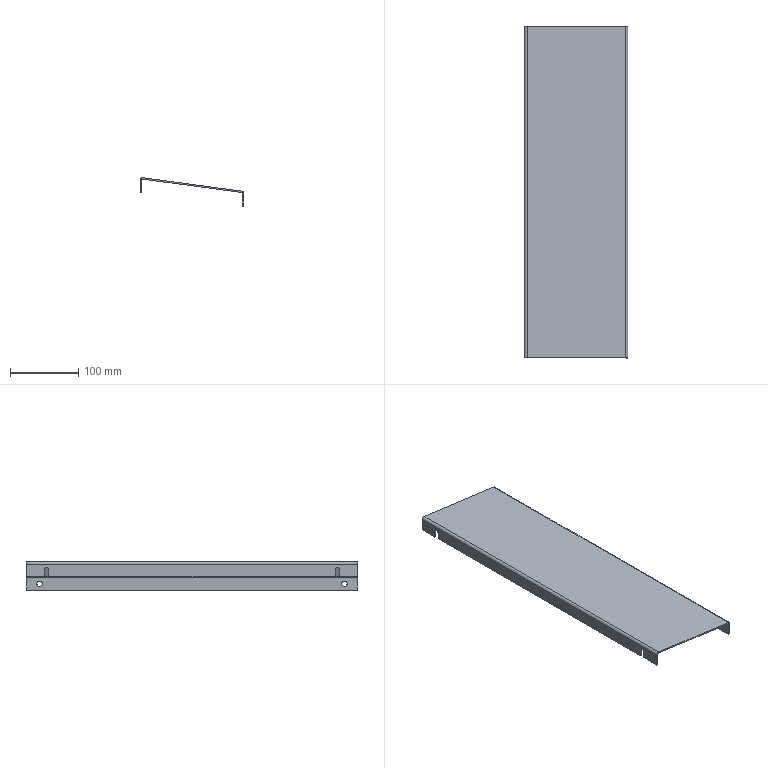Part | STEP file | JBJ-P-1006-08 | 1 solid | 32 faces | box 152 x 488 x 41.784 mm | volume 186030 mm3 | plane 24 | cylinder 8 | commonest cylinder face diameters 3 x2 6.5 x2 7 x2 8 x2
STEP:
#1=CARTESIAN_POINT('',(-2.,461.25,0.));
#2=VERTEX_POINT('',#1);
#3=CARTESIAN_POINT('',(0.,461.25,0.));
#4=VERTEX_POINT('',#3);
#5=CARTESIAN_POINT('',(-2.,461.25,0.));
#6=DIRECTION('',(1.,0.,0.));
#7=VECTOR('',#6,1000.);
#8=LINE('',#5,#7);
#9=EDGE_CURVE('',#2,#4,#8,.T.);
#10=ORIENTED_EDGE('',*,*,#9,.F.);
#11=CARTESIAN_POINT('',(-2.,488.,0.));
#12=VERTEX_POINT('',#11);
#13=CARTESIAN_POINT('',(-2.,488.,0.));
#14=DIRECTION('',(0.,-1.,0.));
#15=VECTOR('',#14,1000.);
#16=LINE('',#13,#15);
#17=EDGE_CURVE('',#12,#2,#16,.T.);
#18=ORIENTED_EDGE('',*,*,#17,.F.);
#19=CARTESIAN_POINT('',(0.,488.,0.));
#20=VERTEX_POINT('',#19);
#21=CARTESIAN_POINT('',(-2.,488.,0.));
#22=DIRECTION('',(1.,0.,0.));
#23=VECTOR('',#22,1000.);
#24=LINE('',#21,#23);
#25=EDGE_CURVE('',#12,#20,#24,.T.);
#26=ORIENTED_EDGE('',*,*,#25,.T.);
#27=CARTESIAN_POINT('',(0.,488.,0.));
#28=DIRECTION('',(0.,-1.,0.));
#29=VECTOR('',#28,1000.);
#30=LINE('',#27,#29);
#31=EDGE_CURVE('',#20,#4,#30,.T.);
#32=ORIENTED_EDGE('',*,*,#31,.T.);
#33=EDGE_LOOP('',(#10,#18,#26,#32));
#34=FACE_OUTER_BOUND('',#33,.T.);
#35=CARTESIAN_POINT('',(-2.,488.,0.));
#36=DIRECTION('',(0.,0.,-1.));
#37=DIRECTION('',(-1.,0.,0.));
#38=AXIS2_PLACEMENT_3D('',#35,#36,#37);
#39=PLANE('',#38);
#40=ADVANCED_FACE('',(#34),#39,.T.);
#41=CARTESIAN_POINT('',(0.,454.75,0.));
#42=VERTEX_POINT('',#41);
#43=CARTESIAN_POINT('',(-2.,454.75,0.));
#44=VERTEX_POINT('',#43);
#45=CARTESIAN_POINT('',(-2.,454.75,0.));
#46=DIRECTION('',(-1.,0.,0.));
#47=VECTOR('',#46,1000.);
#48=LINE('',#45,#47);
#49=EDGE_CURVE('',#42,#44,#48,.T.);
#50=ORIENTED_EDGE('',*,*,#49,.F.);
#51=CARTESIAN_POINT('',(0.,33.25,0.));
#52=VERTEX_POINT('',#51);
#53=CARTESIAN_POINT('',(0.,488.,0.));
#54=DIRECTION('',(0.,-1.,0.));
#55=VECTOR('',#54,1000.);
#56=LINE('',#53,#55);
#57=EDGE_CURVE('',#42,#52,#56,.T.);
#58=ORIENTED_EDGE('',*,*,#57,.T.);
#59=CARTESIAN_POINT('',(-2.,33.25,0.));
#60=VERTEX_POINT('',#59);
#61=CARTESIAN_POINT('',(-2.,33.25,0.));
#62=DIRECTION('',(1.,0.,0.));
#63=VECTOR('',#62,1000.);
#64=LINE('',#61,#63);
#65=EDGE_CURVE('',#60,#52,#64,.T.);
#66=ORIENTED_EDGE('',*,*,#65,.F.);
#67=CARTESIAN_POINT('',(-2.,488.,0.));
#68=DIRECTION('',(0.,-1.,0.));
#69=VECTOR('',#68,1000.);
#70=LINE('',#67,#69);
#71=EDGE_CURVE('',#44,#60,#70,.T.);
#72=ORIENTED_EDGE('',*,*,#71,.F.);
#73=EDGE_LOOP('',(#50,#58,#66,#72));
#74=FACE_OUTER_BOUND('',#73,.T.);
#75=CARTESIAN_POINT('',(-2.,488.,0.));
#76=DIRECTION('',(0.,0.,-1.));
#77=DIRECTION('',(-1.,0.,0.));
#78=AXIS2_PLACEMENT_3D('',#75,#76,#77);
#79=PLANE('',#78);
#80=ADVANCED_FACE('',(#74),#79,.T.);
#81=CARTESIAN_POINT('',(1.701,488.,19.77));
#82=VERTEX_POINT('',#81);
#83=CARTESIAN_POINT('',(1.969,488.,21.752));
#84=VERTEX_POINT('',#83);
#85=CARTESIAN_POINT('',(1.701,488.,19.77));
#86=DIRECTION('',(0.1339,0.,0.991));
#87=VECTOR('',#86,1000.);
#88=LINE('',#85,#87);
#89=EDGE_CURVE('',#82,#84,#88,.T.);
#90=ORIENTED_EDGE('',*,*,#89,.F.);
#91=CARTESIAN_POINT('',(0.,488.,18.284));
#92=VERTEX_POINT('',#91);
#93=CARTESIAN_POINT('',(1.5,488.,18.284));
#94=DIRECTION('',(0.,1.,0.));
#95=DIRECTION('',(0.,0.,-1.));
#96=AXIS2_PLACEMENT_3D('',#93,#94,#95);
#97=CIRCLE('',#96,1.5);
#98=EDGE_CURVE('',#92,#82,#97,.T.);
#99=ORIENTED_EDGE('',*,*,#98,.F.);
#100=CARTESIAN_POINT('',(-2.,488.,18.284));
#101=VERTEX_POINT('',#100);
#102=CARTESIAN_POINT('',(-2.,488.,18.284));
#103=DIRECTION('',(1.,0.,0.));
#104=VECTOR('',#103,1000.);
#105=LINE('',#102,#104);
#106=EDGE_CURVE('',#101,#92,#105,.T.);
#107=ORIENTED_EDGE('',*,*,#106,.F.);
#108=CARTESIAN_POINT('',(1.5,488.,18.284));
#109=DIRECTION('',(0.,1.,0.));
#110=DIRECTION('',(1.,0.,0.));
#111=AXIS2_PLACEMENT_3D('',#108,#109,#110);
#112=CIRCLE('',#111,3.5);
#113=EDGE_CURVE('',#101,#84,#112,.T.);
#114=ORIENTED_EDGE('',*,*,#113,.T.);
#115=EDGE_LOOP('',(#90,#99,#107,#114));
#116=FACE_OUTER_BOUND('',#115,.T.);
#117=CARTESIAN_POINT('',(1.701,488.,19.77));
#118=DIRECTION('',(0.,1.,0.));
#119=DIRECTION('',(0.,0.,1.));
#120=AXIS2_PLACEMENT_3D('',#117,#118,#119);
#121=PLANE('',#120);
#122=ADVANCED_FACE('',(#116),#121,.T.);
#123=CARTESIAN_POINT('',(146.701,488.,0.1756));
#124=VERTEX_POINT('',#123);
#125=CARTESIAN_POINT('',(0.,488.,20.));
#126=DIRECTION('',(0.991,0.,-0.1339));
#127=VECTOR('',#126,1000.);
#128=LINE('',#125,#127);
#129=EDGE_CURVE('',#82,#124,#128,.T.);
#130=ORIENTED_EDGE('',*,*,#129,.F.);
#131=ORIENTED_EDGE('',*,*,#89,.T.);
#132=CARTESIAN_POINT('',(146.969,488.,2.158));
#133=VERTEX_POINT('',#132);
#134=CARTESIAN_POINT('',(0.2678,488.,21.982));
#135=DIRECTION('',(0.991,0.,-0.1339));
#136=VECTOR('',#135,1000.);
#137=LINE('',#134,#136);
#138=EDGE_CURVE('',#84,#133,#137,.T.);
#139=ORIENTED_EDGE('',*,*,#138,.T.);
#140=CARTESIAN_POINT('',(146.969,488.,2.158));
#141=DIRECTION('',(-0.1339,0.,-0.991));
#142=VECTOR('',#141,1000.);
#143=LINE('',#140,#142);
#144=EDGE_CURVE('',#133,#124,#143,.T.);
#145=ORIENTED_EDGE('',*,*,#144,.T.);
#146=EDGE_LOOP('',(#130,#131,#139,#145));
#147=FACE_OUTER_BOUND('',#146,.T.);
#148=CARTESIAN_POINT('',(-2.,488.,18.284));
#149=DIRECTION('',(0.,1.,0.));
#150=DIRECTION('',(0.,0.,1.));
#151=AXIS2_PLACEMENT_3D('',#148,#149,#150);
#152=PLANE('',#151);
#153=ADVANCED_FACE('',(#147),#152,.T.);
#154=CARTESIAN_POINT('',(0.,0.,18.284));
#155=VERTEX_POINT('',#154);
#156=CARTESIAN_POINT('',(-2.,0.,18.284));
#157=VERTEX_POINT('',#156);
#158=CARTESIAN_POINT('',(0.,0.,18.284));
#159=DIRECTION('',(-1.,0.,0.));
#160=VECTOR('',#159,1000.);
#161=LINE('',#158,#160);
#162=EDGE_CURVE('',#155,#157,#161,.T.);
#163=ORIENTED_EDGE('',*,*,#162,.F.);
#164=CARTESIAN_POINT('',(1.701,0.,19.77));
#165=VERTEX_POINT('',#164);
#166=CARTESIAN_POINT('',(1.5,0.,18.284));
#167=DIRECTION('',(0.,1.,0.));
#168=DIRECTION('',(0.,0.,-1.));
#169=AXIS2_PLACEMENT_3D('',#166,#167,#168);
#170=CIRCLE('',#169,1.5);
#171=EDGE_CURVE('',#155,#165,#170,.T.);
#172=ORIENTED_EDGE('',*,*,#171,.T.);
#173=CARTESIAN_POINT('',(1.969,0.,21.752));
#174=VERTEX_POINT('',#173);
#175=CARTESIAN_POINT('',(1.969,0.,21.752));
#176=DIRECTION('',(-0.1339,0.,-0.991));
#177=VECTOR('',#176,1000.);
#178=LINE('',#175,#177);
#179=EDGE_CURVE('',#174,#165,#178,.T.);
#180=ORIENTED_EDGE('',*,*,#179,.F.);
#181=CARTESIAN_POINT('',(1.5,0.,18.284));
#182=DIRECTION('',(0.,1.,0.));
#183=DIRECTION('',(1.,0.,0.));
#184=AXIS2_PLACEMENT_3D('',#181,#182,#183);
#185=CIRCLE('',#184,3.5);
#186=EDGE_CURVE('',#157,#174,#185,.T.);
#187=ORIENTED_EDGE('',*,*,#186,.F.);
#188=EDGE_LOOP('',(#163,#172,#180,#187));
#189=FACE_OUTER_BOUND('',#188,.T.);
#190=CARTESIAN_POINT('',(0.,0.,18.284));
#191=DIRECTION('',(0.,-1.,0.));
#192=DIRECTION('',(0.,0.,-1.));
#193=AXIS2_PLACEMENT_3D('',#190,#191,#192);
#194=PLANE('',#193);
#195=ADVANCED_FACE('',(#189),#194,.T.);
#196=CARTESIAN_POINT('',(0.,0.,0.));
#197=VERTEX_POINT('',#196);
#198=CARTESIAN_POINT('',(0.,0.,0.));
#199=DIRECTION('',(0.,0.,1.));
#200=VECTOR('',#199,1000.);
#201=LINE('',#198,#200);
#202=EDGE_CURVE('',#197,#155,#201,.T.);
#203=ORIENTED_EDGE('',*,*,#202,.T.);
#204=ORIENTED_EDGE('',*,*,#162,.T.);
#205=CARTESIAN_POINT('',(-2.,0.,0.));
#206=VERTEX_POINT('',#205);
#207=CARTESIAN_POINT('',(-2.,0.,0.));
#208=DIRECTION('',(0.,0.,1.));
#209=VECTOR('',#208,1000.);
#210=LINE('',#207,#209);
#211=EDGE_CURVE('',#206,#157,#210,.T.);
#212=ORIENTED_EDGE('',*,*,#211,.F.);
#213=CARTESIAN_POINT('',(-2.,0.,0.));
#214=DIRECTION('',(1.,0.,0.));
#215=VECTOR('',#214,1000.);
#216=LINE('',#213,#215);
#217=EDGE_CURVE('',#206,#197,#216,.T.);
#218=ORIENTED_EDGE('',*,*,#217,.T.);
#219=EDGE_LOOP('',(#203,#204,#212,#218));
#220=FACE_OUTER_BOUND('',#219,.T.);
#221=CARTESIAN_POINT('',(1.969,0.,21.752));
#222=DIRECTION('',(0.,-1.,0.));
#223=DIRECTION('',(0.,0.,-1.));
#224=AXIS2_PLACEMENT_3D('',#221,#222,#223);
#225=PLANE('',#224);
#226=ADVANCED_FACE('',(#220),#225,.T.);
#227=CARTESIAN_POINT('',(148.,488.,-1.311));
#228=VERTEX_POINT('',#227);
#229=CARTESIAN_POINT('',(150.,488.,-1.311));
#230=VERTEX_POINT('',#229);
#231=CARTESIAN_POINT('',(148.,488.,-1.311));
#232=DIRECTION('',(1.,0.,0.));
#233=VECTOR('',#232,1000.);
#234=LINE('',#231,#233);
#235=EDGE_CURVE('',#228,#230,#234,.T.);
#236=ORIENTED_EDGE('',*,*,#235,.F.);
#237=CARTESIAN_POINT('',(146.5,488.,-1.311));
#238=DIRECTION('',(0.,1.,0.));
#239=DIRECTION('',(0.,0.,-1.));
#240=AXIS2_PLACEMENT_3D('',#237,#238,#239);
#241=CIRCLE('',#240,1.5);
#242=EDGE_CURVE('',#124,#228,#241,.T.);
#243=ORIENTED_EDGE('',*,*,#242,.F.);
#244=ORIENTED_EDGE('',*,*,#144,.F.);
#245=CARTESIAN_POINT('',(146.5,488.,-1.311));
#246=DIRECTION('',(0.,1.,0.));
#247=DIRECTION('',(1.,0.,0.));
#248=AXIS2_PLACEMENT_3D('',#245,#246,#247);
#249=CIRCLE('',#248,3.5);
#250=EDGE_CURVE('',#133,#230,#249,.T.);
#251=ORIENTED_EDGE('',*,*,#250,.T.);
#252=EDGE_LOOP('',(#236,#243,#244,#251));
#253=FACE_OUTER_BOUND('',#252,.T.);
#254=CARTESIAN_POINT('',(148.,488.,-1.311));
#255=DIRECTION('',(0.,1.,0.));
#256=DIRECTION('',(0.,0.,1.));
#257=AXIS2_PLACEMENT_3D('',#254,#255,#256);
#258=PLANE('',#257);
#259=ADVANCED_FACE('',(#253),#258,.T.);
#260=CARTESIAN_POINT('',(148.,488.,-20.));
#261=VERTEX_POINT('',#260);
#262=CARTESIAN_POINT('',(148.,488.,0.));
#263=DIRECTION('',(0.,0.,-1.));
#264=VECTOR('',#263,1000.);
#265=LINE('',#262,#264);
#266=EDGE_CURVE('',#228,#261,#265,.T.);
#267=ORIENTED_EDGE('',*,*,#266,.F.);
#268=ORIENTED_EDGE('',*,*,#235,.T.);
#269=CARTESIAN_POINT('',(150.,488.,-20.));
#270=VERTEX_POINT('',#269);
#271=CARTESIAN_POINT('',(150.,488.,0.));
#272=DIRECTION('',(0.,0.,-1.));
#273=VECTOR('',#272,1000.);
#274=LINE('',#271,#273);
#275=EDGE_CURVE('',#230,#270,#274,.T.);
#276=ORIENTED_EDGE('',*,*,#275,.T.);
#277=CARTESIAN_POINT('',(148.,488.,-20.));
#278=DIRECTION('',(1.,0.,0.));
#279=VECTOR('',#278,1000.);
#280=LINE('',#277,#279);
#281=EDGE_CURVE('',#261,#270,#280,.T.);
#282=ORIENTED_EDGE('',*,*,#281,.F.);
#283=EDGE_LOOP('',(#267,#268,#276,#282));
#284=FACE_OUTER_BOUND('',#283,.T.);
#285=CARTESIAN_POINT('',(146.969,488.,2.158));
#286=DIRECTION('',(0.,1.,0.));
#287=DIRECTION('',(0.,0.,1.));
#288=AXIS2_PLACEMENT_3D('',#285,#286,#287);
#289=PLANE('',#288);
#290=ADVANCED_FACE('',(#284),#289,.T.);
#291=CARTESIAN_POINT('',(146.701,0.,0.1756));
#292=VERTEX_POINT('',#291);
#293=CARTESIAN_POINT('',(146.969,0.,2.158));
#294=VERTEX_POINT('',#293);
#295=CARTESIAN_POINT('',(146.701,0.,0.1756));
#296=DIRECTION('',(0.1339,0.,0.991));
#297=VECTOR('',#296,1000.);
#298=LINE('',#295,#297);
#299=EDGE_CURVE('',#292,#294,#298,.T.);
#300=ORIENTED_EDGE('',*,*,#299,.F.);
#301=CARTESIAN_POINT('',(148.,0.,-1.311));
#302=VERTEX_POINT('',#301);
#303=CARTESIAN_POINT('',(146.5,0.,-1.311));
#304=DIRECTION('',(0.,1.,0.));
#305=DIRECTION('',(0.,0.,-1.));
#306=AXIS2_PLACEMENT_3D('',#303,#304,#305);
#307=CIRCLE('',#306,1.5);
#308=EDGE_CURVE('',#292,#302,#307,.T.);
#309=ORIENTED_EDGE('',*,*,#308,.T.);
#310=CARTESIAN_POINT('',(150.,0.,-1.311));
#311=VERTEX_POINT('',#310);
#312=CARTESIAN_POINT('',(150.,0.,-1.311));
#313=DIRECTION('',(-1.,0.,0.));
#314=VECTOR('',#313,1000.);
#315=LINE('',#312,#314);
#316=EDGE_CURVE('',#311,#302,#315,.T.);
#317=ORIENTED_EDGE('',*,*,#316,.F.);
#318=CARTESIAN_POINT('',(146.5,0.,-1.311));
#319=DIRECTION('',(0.,1.,0.));
#320=DIRECTION('',(1.,0.,0.));
#321=AXIS2_PLACEMENT_3D('',#318,#319,#320);
#322=CIRCLE('',#321,3.5);
#323=EDGE_CURVE('',#294,#311,#322,.T.);
#324=ORIENTED_EDGE('',*,*,#323,.F.);
#325=EDGE_LOOP('',(#300,#309,#317,#324));
#326=FACE_OUTER_BOUND('',#325,.T.);
#327=CARTESIAN_POINT('',(146.701,0.,0.1756));
#328=DIRECTION('',(0.,-1.,0.));
#329=DIRECTION('',(0.,0.,-1.));
#330=AXIS2_PLACEMENT_3D('',#327,#328,#329);
#331=PLANE('',#330);
#332=ADVANCED_FACE('',(#326),#331,.T.);
#333=CARTESIAN_POINT('',(0.,0.,20.));
#334=DIRECTION('',(0.991,0.,-0.1339));
#335=VECTOR('',#334,1000.);
#336=LINE('',#333,#335);
#337=EDGE_CURVE('',#165,#292,#336,.T.);
#338=ORIENTED_EDGE('',*,*,#337,.T.);
#339=ORIENTED_EDGE('',*,*,#299,.T.);
#340=CARTESIAN_POINT('',(0.2678,0.,21.982));
#341=DIRECTION('',(0.991,0.,-0.1339));
#342=VECTOR('',#341,1000.);
#343=LINE('',#340,#342);
#344=EDGE_CURVE('',#174,#294,#343,.T.);
#345=ORIENTED_EDGE('',*,*,#344,.F.);
#346=ORIENTED_EDGE('',*,*,#179,.T.);
#347=EDGE_LOOP('',(#338,#339,#345,#346));
#348=FACE_OUTER_BOUND('',#347,.T.);
#349=CARTESIAN_POINT('',(150.,0.,-1.311));
#350=DIRECTION('',(0.,-1.,0.));
#351=DIRECTION('',(0.,0.,-1.));
#352=AXIS2_PLACEMENT_3D('',#349,#350,#351);
#353=PLANE('',#352);
#354=ADVANCED_FACE('',(#348),#353,.T.);
#355=CARTESIAN_POINT('',(150.,468.,-6.655));
#356=VERTEX_POINT('',#355);
#357=CARTESIAN_POINT('',(150.,468.,-10.655));
#358=DIRECTION('',(-1.,0.,0.));
#359=DIRECTION('',(0.,0.,1.));
#360=AXIS2_PLACEMENT_3D('',#357,#358,#359);
#361=CIRCLE('',#360,4.);
#362=EDGE_CURVE('',#356,#356,#361,.T.);
#363=ORIENTED_EDGE('',*,*,#362,.T.);
#364=EDGE_LOOP('',(#363));
#365=FACE_BOUND('',#364,.T.);
#366=CARTESIAN_POINT('',(150.,20.,-6.655));
#367=VERTEX_POINT('',#366);
#368=CARTESIAN_POINT('',(150.,20.,-10.655));
#369=DIRECTION('',(-1.,0.,0.));
#370=DIRECTION('',(0.,0.,1.));
#371=AXIS2_PLACEMENT_3D('',#368,#369,#370);
#372=CIRCLE('',#371,4.);
#373=EDGE_CURVE('',#367,#367,#372,.T.);
#374=ORIENTED_EDGE('',*,*,#373,.T.);
#375=EDGE_LOOP('',(#374));
#376=FACE_BOUND('',#375,.T.);
#377=CARTESIAN_POINT('',(150.,0.,-20.));
#378=VERTEX_POINT('',#377);
#379=CARTESIAN_POINT('',(150.,0.,0.));
#380=DIRECTION('',(0.,0.,-1.));
#381=VECTOR('',#380,1000.);
#382=LINE('',#379,#381);
#383=EDGE_CURVE('',#311,#378,#382,.T.);
#384=ORIENTED_EDGE('',*,*,#383,.T.);
#385=CARTESIAN_POINT('',(150.,488.,-20.));
#386=DIRECTION('',(0.,-1.,0.));
#387=VECTOR('',#386,1000.);
#388=LINE('',#385,#387);
#389=EDGE_CURVE('',#270,#378,#388,.T.);
#390=ORIENTED_EDGE('',*,*,#389,.F.);
#391=ORIENTED_EDGE('',*,*,#275,.F.);
#392=CARTESIAN_POINT('',(150.,488.,-1.311));
#393=DIRECTION('',(0.,-1.,0.));
#394=VECTOR('',#393,1000.);
#395=LINE('',#392,#394);
#396=EDGE_CURVE('',#230,#311,#395,.T.);
#397=ORIENTED_EDGE('',*,*,#396,.T.);
#398=EDGE_LOOP('',(#384,#390,#391,#397));
#399=FACE_OUTER_BOUND('',#398,.T.);
#400=CARTESIAN_POINT('',(150.,488.,0.));
#401=DIRECTION('',(-1.,0.,0.));
#402=DIRECTION('',(0.,0.,1.));
#403=AXIS2_PLACEMENT_3D('',#400,#401,#402);
#404=PLANE('',#403);
#405=ADVANCED_FACE('',(#365,#376,#399),#404,.F.);
#406=CARTESIAN_POINT('',(148.,0.,-20.));
#407=VERTEX_POINT('',#406);
#408=CARTESIAN_POINT('',(148.,0.,-20.));
#409=DIRECTION('',(1.,0.,0.));
#410=VECTOR('',#409,1000.);
#411=LINE('',#408,#410);
#412=EDGE_CURVE('',#407,#378,#411,.T.);
#413=ORIENTED_EDGE('',*,*,#412,.F.);
#414=CARTESIAN_POINT('',(148.,488.,-20.));
#415=DIRECTION('',(0.,-1.,0.));
#416=VECTOR('',#415,1000.);
#417=LINE('',#414,#416);
#418=EDGE_CURVE('',#261,#407,#417,.T.);
#419=ORIENTED_EDGE('',*,*,#418,.F.);
#420=ORIENTED_EDGE('',*,*,#281,.T.);
#421=ORIENTED_EDGE('',*,*,#389,.T.);
#422=EDGE_LOOP('',(#413,#419,#420,#421));
#423=FACE_OUTER_BOUND('',#422,.T.);
#424=CARTESIAN_POINT('',(148.,488.,-20.));
#425=DIRECTION('',(0.,0.,-1.));
#426=DIRECTION('',(-1.,0.,0.));
#427=AXIS2_PLACEMENT_3D('',#424,#425,#426);
#428=PLANE('',#427);
#429=ADVANCED_FACE('',(#423),#428,.T.);
#430=CARTESIAN_POINT('',(148.,468.,-6.655));
#431=VERTEX_POINT('',#430);
#432=CARTESIAN_POINT('',(148.,468.,-10.655));
#433=DIRECTION('',(-1.,0.,0.));
#434=DIRECTION('',(0.,0.,1.));
#435=AXIS2_PLACEMENT_3D('',#432,#433,#434);
#436=CIRCLE('',#435,4.);
#437=EDGE_CURVE('',#431,#431,#436,.T.);
#438=ORIENTED_EDGE('',*,*,#437,.F.);
#439=EDGE_LOOP('',(#438));
#440=FACE_BOUND('',#439,.T.);
#441=CARTESIAN_POINT('',(148.,20.,-6.655));
#442=VERTEX_POINT('',#441);
#443=CARTESIAN_POINT('',(148.,20.,-10.655));
#444=DIRECTION('',(-1.,0.,0.));
#445=DIRECTION('',(0.,0.,1.));
#446=AXIS2_PLACEMENT_3D('',#443,#444,#445);
#447=CIRCLE('',#446,4.);
#448=EDGE_CURVE('',#442,#442,#447,.T.);
#449=ORIENTED_EDGE('',*,*,#448,.F.);
#450=EDGE_LOOP('',(#449));
#451=FACE_BOUND('',#450,.T.);
#452=CARTESIAN_POINT('',(148.,0.,0.));
#453=DIRECTION('',(0.,0.,-1.));
#454=VECTOR('',#453,1000.);
#455=LINE('',#452,#454);
#456=EDGE_CURVE('',#302,#407,#455,.T.);
#457=ORIENTED_EDGE('',*,*,#456,.F.);
#458=CARTESIAN_POINT('',(148.,488.,-1.311));
#459=DIRECTION('',(0.,-1.,0.));
#460=VECTOR('',#459,1000.);
#461=LINE('',#458,#460);
#462=EDGE_CURVE('',#228,#302,#461,.T.);
#463=ORIENTED_EDGE('',*,*,#462,.F.);
#464=ORIENTED_EDGE('',*,*,#266,.T.);
#465=ORIENTED_EDGE('',*,*,#418,.T.);
#466=EDGE_LOOP('',(#457,#463,#464,#465));
#467=FACE_OUTER_BOUND('',#466,.T.);
#468=CARTESIAN_POINT('',(148.,488.,0.));
#469=DIRECTION('',(-1.,0.,0.));
#470=DIRECTION('',(0.,0.,1.));
#471=AXIS2_PLACEMENT_3D('',#468,#469,#470);
#472=PLANE('',#471);
#473=ADVANCED_FACE('',(#440,#451,#467),#472,.T.);
#474=ORIENTED_EDGE('',*,*,#308,.F.);
#475=CARTESIAN_POINT('',(146.701,488.,0.1756));
#476=DIRECTION('',(0.,-1.,0.));
#477=VECTOR('',#476,1000.);
#478=LINE('',#475,#477);
#479=EDGE_CURVE('',#124,#292,#478,.T.);
#480=ORIENTED_EDGE('',*,*,#479,.F.);
#481=ORIENTED_EDGE('',*,*,#242,.T.);
#482=ORIENTED_EDGE('',*,*,#462,.T.);
#483=EDGE_LOOP('',(#474,#480,#481,#482));
#484=FACE_OUTER_BOUND('',#483,.T.);
#485=CARTESIAN_POINT('',(146.5,488.,-1.311));
#486=DIRECTION('',(0.,-1.,0.));
#487=DIRECTION('',(0.,0.,-1.));
#488=AXIS2_PLACEMENT_3D('',#485,#486,#487);
#489=CYLINDRICAL_SURFACE('',#488,1.5);
#490=ADVANCED_FACE('',(#484),#489,.F.);
#491=ORIENTED_EDGE('',*,*,#337,.F.);
#492=CARTESIAN_POINT('',(1.701,488.,19.77));
#493=DIRECTION('',(0.,-1.,0.));
#494=VECTOR('',#493,1000.);
#495=LINE('',#492,#494);
#496=EDGE_CURVE('',#82,#165,#495,.T.);
#497=ORIENTED_EDGE('',*,*,#496,.F.);
#498=ORIENTED_EDGE('',*,*,#129,.T.);
#499=ORIENTED_EDGE('',*,*,#479,.T.);
#500=EDGE_LOOP('',(#491,#497,#498,#499));
#501=FACE_OUTER_BOUND('',#500,.T.);
#502=CARTESIAN_POINT('',(0.,488.,20.));
#503=DIRECTION('',(-0.1339,0.,-0.991));
#504=DIRECTION('',(-0.991,0.,0.1339));
#505=AXIS2_PLACEMENT_3D('',#502,#503,#504);
#506=PLANE('',#505);
#507=ADVANCED_FACE('',(#501),#506,.T.);
#508=ORIENTED_EDGE('',*,*,#171,.F.);
#509=CARTESIAN_POINT('',(0.,488.,18.284));
#510=DIRECTION('',(0.,-1.,0.));
#511=VECTOR('',#510,1000.);
#512=LINE('',#509,#511);
#513=EDGE_CURVE('',#92,#155,#512,.T.);
#514=ORIENTED_EDGE('',*,*,#513,.F.);
#515=ORIENTED_EDGE('',*,*,#98,.T.);
#516=ORIENTED_EDGE('',*,*,#496,.T.);
#517=EDGE_LOOP('',(#508,#514,#515,#516));
#518=FACE_OUTER_BOUND('',#517,.T.);
#519=CARTESIAN_POINT('',(1.5,488.,18.284));
#520=DIRECTION('',(0.,-1.,0.));
#521=DIRECTION('',(0.,0.,-1.));
#522=AXIS2_PLACEMENT_3D('',#519,#520,#521);
#523=CYLINDRICAL_SURFACE('',#522,1.5);
#524=ADVANCED_FACE('',(#518),#523,.F.);
#525=CARTESIAN_POINT('',(0.,461.25,10.));
#526=VERTEX_POINT('',#525);
#527=CARTESIAN_POINT('',(0.,461.25,10.));
#528=DIRECTION('',(0.,0.,1.));
#529=VECTOR('',#528,1000.);
#530=LINE('',#527,#529);
#531=EDGE_CURVE('',#4,#526,#530,.T.);
#532=ORIENTED_EDGE('',*,*,#531,.F.);
#533=ORIENTED_EDGE('',*,*,#31,.F.);
#534=CARTESIAN_POINT('',(0.,488.,0.));
#535=DIRECTION('',(0.,0.,1.));
#536=VECTOR('',#535,1000.);
#537=LINE('',#534,#536);
#538=EDGE_CURVE('',#20,#92,#537,.T.);
#539=ORIENTED_EDGE('',*,*,#538,.T.);
#540=ORIENTED_EDGE('',*,*,#513,.T.);
#541=ORIENTED_EDGE('',*,*,#202,.F.);
#542=CARTESIAN_POINT('',(0.,26.75,0.));
#543=VERTEX_POINT('',#542);
#544=CARTESIAN_POINT('',(0.,488.,0.));
#545=DIRECTION('',(0.,-1.,0.));
#546=VECTOR('',#545,1000.);
#547=LINE('',#544,#546);
#548=EDGE_CURVE('',#543,#197,#547,.T.);
#549=ORIENTED_EDGE('',*,*,#548,.F.);
#550=CARTESIAN_POINT('',(0.,26.75,10.));
#551=VERTEX_POINT('',#550);
#552=CARTESIAN_POINT('',(0.,26.75,10.));
#553=DIRECTION('',(0.,0.,-1.));
#554=VECTOR('',#553,1000.);
#555=LINE('',#552,#554);
#556=EDGE_CURVE('',#551,#543,#555,.T.);
#557=ORIENTED_EDGE('',*,*,#556,.F.);
#558=CARTESIAN_POINT('',(0.,33.25,10.));
#559=VERTEX_POINT('',#558);
#560=CARTESIAN_POINT('',(0.,30.,10.));
#561=DIRECTION('',(1.,0.,0.));
#562=DIRECTION('',(0.,0.,1.));
#563=AXIS2_PLACEMENT_3D('',#560,#561,#562);
#564=CIRCLE('',#563,3.25);
#565=EDGE_CURVE('',#559,#551,#564,.T.);
#566=ORIENTED_EDGE('',*,*,#565,.F.);
#567=CARTESIAN_POINT('',(0.,33.25,10.));
#568=DIRECTION('',(0.,0.,1.));
#569=VECTOR('',#568,1000.);
#570=LINE('',#567,#569);
#571=EDGE_CURVE('',#52,#559,#570,.T.);
#572=ORIENTED_EDGE('',*,*,#571,.F.);
#573=ORIENTED_EDGE('',*,*,#57,.F.);
#574=CARTESIAN_POINT('',(0.,454.75,10.));
#575=VERTEX_POINT('',#574);
#576=CARTESIAN_POINT('',(0.,454.75,10.));
#577=DIRECTION('',(0.,0.,-1.));
#578=VECTOR('',#577,1000.);
#579=LINE('',#576,#578);
#580=EDGE_CURVE('',#575,#42,#579,.T.);
#581=ORIENTED_EDGE('',*,*,#580,.F.);
#582=CARTESIAN_POINT('',(0.,458.,10.));
#583=DIRECTION('',(1.,0.,0.));
#584=DIRECTION('',(0.,0.,-1.));
#585=AXIS2_PLACEMENT_3D('',#582,#583,#584);
#586=CIRCLE('',#585,3.25);
#587=EDGE_CURVE('',#526,#575,#586,.T.);
#588=ORIENTED_EDGE('',*,*,#587,.F.);
#589=EDGE_LOOP('',(#532,#533,#539,#540,#541,#549,#557,#566,#572,#573,#581,#588));
#590=FACE_OUTER_BOUND('',#589,.T.);
#591=CARTESIAN_POINT('',(0.,488.,0.));
#592=DIRECTION('',(1.,0.,0.));
#593=DIRECTION('',(0.,0.,-1.));
#594=AXIS2_PLACEMENT_3D('',#591,#592,#593);
#595=PLANE('',#594);
#596=ADVANCED_FACE('',(#590),#595,.T.);
#597=CARTESIAN_POINT('',(-2.,26.75,0.));
#598=VERTEX_POINT('',#597);
#599=CARTESIAN_POINT('',(-2.,26.75,0.));
#600=DIRECTION('',(-1.,0.,0.));
#601=VECTOR('',#600,1000.);
#602=LINE('',#599,#601);
#603=EDGE_CURVE('',#543,#598,#602,.T.);
#604=ORIENTED_EDGE('',*,*,#603,.F.);
#605=ORIENTED_EDGE('',*,*,#548,.T.);
#606=ORIENTED_EDGE('',*,*,#217,.F.);
#607=CARTESIAN_POINT('',(-2.,488.,0.));
#608=DIRECTION('',(0.,-1.,0.));
#609=VECTOR('',#608,1000.);
#610=LINE('',#607,#609);
#611=EDGE_CURVE('',#598,#206,#610,.T.);
#612=ORIENTED_EDGE('',*,*,#611,.F.);
#613=EDGE_LOOP('',(#604,#605,#606,#612));
#614=FACE_OUTER_BOUND('',#613,.T.);
#615=CARTESIAN_POINT('',(-2.,488.,0.));
#616=DIRECTION('',(0.,0.,-1.));
#617=DIRECTION('',(-1.,0.,0.));
#618=AXIS2_PLACEMENT_3D('',#615,#616,#617);
#619=PLANE('',#618);
#620=ADVANCED_FACE('',(#614),#619,.T.);
#621=ORIENTED_EDGE('',*,*,#17,.T.);
#622=CARTESIAN_POINT('',(-2.,461.25,10.));
#623=VERTEX_POINT('',#622);
#624=CARTESIAN_POINT('',(-2.,461.25,0.));
#625=DIRECTION('',(0.,0.,1.));
#626=VECTOR('',#625,1000.);
#627=LINE('',#624,#626);
#628=EDGE_CURVE('',#2,#623,#627,.T.);
#629=ORIENTED_EDGE('',*,*,#628,.T.);
#630=CARTESIAN_POINT('',(-2.,454.75,10.));
#631=VERTEX_POINT('',#630);
#632=CARTESIAN_POINT('',(-2.,458.,10.));
#633=DIRECTION('',(1.,0.,0.));
#634=DIRECTION('',(0.,0.,-1.));
#635=AXIS2_PLACEMENT_3D('',#632,#633,#634);
#636=CIRCLE('',#635,3.25);
#637=EDGE_CURVE('',#623,#631,#636,.T.);
#638=ORIENTED_EDGE('',*,*,#637,.T.);
#639=CARTESIAN_POINT('',(-2.,454.75,0.));
#640=DIRECTION('',(0.,0.,-1.));
#641=VECTOR('',#640,1000.);
#642=LINE('',#639,#641);
#643=EDGE_CURVE('',#631,#44,#642,.T.);
#644=ORIENTED_EDGE('',*,*,#643,.T.);
#645=ORIENTED_EDGE('',*,*,#71,.T.);
#646=CARTESIAN_POINT('',(-2.,33.25,10.));
#647=VERTEX_POINT('',#646);
#648=CARTESIAN_POINT('',(-2.,33.25,0.));
#649=DIRECTION('',(0.,0.,1.));
#650=VECTOR('',#649,1000.);
#651=LINE('',#648,#650);
#652=EDGE_CURVE('',#60,#647,#651,.T.);
#653=ORIENTED_EDGE('',*,*,#652,.T.);
#654=CARTESIAN_POINT('',(-2.,26.75,10.));
#655=VERTEX_POINT('',#654);
#656=CARTESIAN_POINT('',(-2.,30.,10.));
#657=DIRECTION('',(1.,0.,0.));
#658=DIRECTION('',(0.,0.,-1.));
#659=AXIS2_PLACEMENT_3D('',#656,#657,#658);
#660=CIRCLE('',#659,3.25);
#661=EDGE_CURVE('',#647,#655,#660,.T.);
#662=ORIENTED_EDGE('',*,*,#661,.T.);
#663=CARTESIAN_POINT('',(-2.,26.75,0.));
#664=DIRECTION('',(0.,0.,-1.));
#665=VECTOR('',#664,1000.);
#666=LINE('',#663,#665);
#667=EDGE_CURVE('',#655,#598,#666,.T.);
#668=ORIENTED_EDGE('',*,*,#667,.T.);
#669=ORIENTED_EDGE('',*,*,#611,.T.);
#670=ORIENTED_EDGE('',*,*,#211,.T.);
#671=CARTESIAN_POINT('',(-2.,488.,18.284));
#672=DIRECTION('',(0.,-1.,0.));
#673=VECTOR('',#672,1000.);
#674=LINE('',#671,#673);
#675=EDGE_CURVE('',#101,#157,#674,.T.);
#676=ORIENTED_EDGE('',*,*,#675,.F.);
#677=CARTESIAN_POINT('',(-2.,488.,0.));
#678=DIRECTION('',(0.,0.,1.));
#679=VECTOR('',#678,1000.);
#680=LINE('',#677,#679);
#681=EDGE_CURVE('',#12,#101,#680,.T.);
#682=ORIENTED_EDGE('',*,*,#681,.F.);
#683=EDGE_LOOP('',(#621,#629,#638,#644,#645,#653,#662,#668,#669,#670,#676,#682));
#684=FACE_OUTER_BOUND('',#683,.T.);
#685=CARTESIAN_POINT('',(-2.,488.,0.));
#686=DIRECTION('',(1.,0.,0.));
#687=DIRECTION('',(0.,0.,-1.));
#688=AXIS2_PLACEMENT_3D('',#685,#686,#687);
#689=PLANE('',#688);
#690=ADVANCED_FACE('',(#684),#689,.F.);
#691=ORIENTED_EDGE('',*,*,#186,.T.);
#692=CARTESIAN_POINT('',(1.969,488.,21.752));
#693=DIRECTION('',(0.,-1.,0.));
#694=VECTOR('',#693,1000.);
#695=LINE('',#692,#694);
#696=EDGE_CURVE('',#84,#174,#695,.T.);
#697=ORIENTED_EDGE('',*,*,#696,.F.);
#698=ORIENTED_EDGE('',*,*,#113,.F.);
#699=ORIENTED_EDGE('',*,*,#675,.T.);
#700=EDGE_LOOP('',(#691,#697,#698,#699));
#701=FACE_OUTER_BOUND('',#700,.T.);
#702=CARTESIAN_POINT('',(1.5,488.,18.284));
#703=DIRECTION('',(0.,-1.,0.));
#704=DIRECTION('',(0.,0.,-1.));
#705=AXIS2_PLACEMENT_3D('',#702,#703,#704);
#706=CYLINDRICAL_SURFACE('',#705,3.5);
#707=ADVANCED_FACE('',(#701),#706,.T.);
#708=ORIENTED_EDGE('',*,*,#344,.T.);
#709=CARTESIAN_POINT('',(146.969,488.,2.158));
#710=DIRECTION('',(0.,-1.,0.));
#711=VECTOR('',#710,1000.);
#712=LINE('',#709,#711);
#713=EDGE_CURVE('',#133,#294,#712,.T.);
#714=ORIENTED_EDGE('',*,*,#713,.F.);
#715=ORIENTED_EDGE('',*,*,#138,.F.);
#716=ORIENTED_EDGE('',*,*,#696,.T.);
#717=EDGE_LOOP('',(#708,#714,#715,#716));
#718=FACE_OUTER_BOUND('',#717,.T.);
#719=CARTESIAN_POINT('',(0.2678,488.,21.982));
#720=DIRECTION('',(-0.1339,0.,-0.991));
#721=DIRECTION('',(-0.991,0.,0.1339));
#722=AXIS2_PLACEMENT_3D('',#719,#720,#721);
#723=PLANE('',#722);
#724=ADVANCED_FACE('',(#718),#723,.F.);
#725=ORIENTED_EDGE('',*,*,#323,.T.);
#726=ORIENTED_EDGE('',*,*,#396,.F.);
#727=ORIENTED_EDGE('',*,*,#250,.F.);
#728=ORIENTED_EDGE('',*,*,#713,.T.);
#729=EDGE_LOOP('',(#725,#726,#727,#728));
#730=FACE_OUTER_BOUND('',#729,.T.);
#731=CARTESIAN_POINT('',(146.5,488.,-1.311));
#732=DIRECTION('',(0.,-1.,0.));
#733=DIRECTION('',(0.,0.,-1.));
#734=AXIS2_PLACEMENT_3D('',#731,#732,#733);
#735=CYLINDRICAL_SURFACE('',#734,3.5);
#736=ADVANCED_FACE('',(#730),#735,.T.);
#737=ORIENTED_EDGE('',*,*,#681,.T.);
#738=ORIENTED_EDGE('',*,*,#106,.T.);
#739=ORIENTED_EDGE('',*,*,#538,.F.);
#740=ORIENTED_EDGE('',*,*,#25,.F.);
#741=EDGE_LOOP('',(#737,#738,#739,#740));
#742=FACE_OUTER_BOUND('',#741,.T.);
#743=CARTESIAN_POINT('',(146.5,488.,-1.311));
#744=DIRECTION('',(0.,-1.,0.));
#745=DIRECTION('',(-1.,0.,0.));
#746=AXIS2_PLACEMENT_3D('',#743,#744,#745);
#747=PLANE('',#746);
#748=ADVANCED_FACE('',(#742),#747,.F.);
#749=ORIENTED_EDGE('',*,*,#383,.F.);
#750=ORIENTED_EDGE('',*,*,#316,.T.);
#751=ORIENTED_EDGE('',*,*,#456,.T.);
#752=ORIENTED_EDGE('',*,*,#412,.T.);
#753=EDGE_LOOP('',(#749,#750,#751,#752));
#754=FACE_OUTER_BOUND('',#753,.T.);
#755=CARTESIAN_POINT('',(146.5,0.,-1.311));
#756=DIRECTION('',(0.,-1.,0.));
#757=DIRECTION('',(-1.,0.,0.));
#758=AXIS2_PLACEMENT_3D('',#755,#756,#757);
#759=PLANE('',#758);
#760=ADVANCED_FACE('',(#754),#759,.T.);
#761=ORIENTED_EDGE('',*,*,#448,.T.);
#762=EDGE_LOOP('',(#761));
#763=FACE_OUTER_BOUND('',#762,.T.);
#764=ORIENTED_EDGE('',*,*,#373,.F.);
#765=EDGE_LOOP('',(#764));
#766=FACE_OUTER_BOUND('',#765,.T.);
#767=CARTESIAN_POINT('',(158.,20.,-10.655));
#768=DIRECTION('',(-1.,0.,0.));
#769=DIRECTION('',(0.,0.,1.));
#770=AXIS2_PLACEMENT_3D('',#767,#768,#769);
#771=CYLINDRICAL_SURFACE('',#770,4.);
#772=ADVANCED_FACE('',(#763,#766),#771,.F.);
#773=ORIENTED_EDGE('',*,*,#437,.T.);
#774=EDGE_LOOP('',(#773));
#775=FACE_OUTER_BOUND('',#774,.T.);
#776=ORIENTED_EDGE('',*,*,#362,.F.);
#777=EDGE_LOOP('',(#776));
#778=FACE_OUTER_BOUND('',#777,.T.);
#779=CARTESIAN_POINT('',(158.,468.,-10.655));
#780=DIRECTION('',(-1.,0.,0.));
#781=DIRECTION('',(0.,0.,1.));
#782=AXIS2_PLACEMENT_3D('',#779,#780,#781);
#783=CYLINDRICAL_SURFACE('',#782,4.);
#784=ADVANCED_FACE('',(#775,#778),#783,.F.);
#785=CARTESIAN_POINT('',(-10.,33.25,10.));
#786=DIRECTION('',(1.,0.,0.));
#787=VECTOR('',#786,1000.);
#788=LINE('',#785,#787);
#789=EDGE_CURVE('',#647,#559,#788,.T.);
#790=ORIENTED_EDGE('',*,*,#789,.T.);
#791=ORIENTED_EDGE('',*,*,#565,.T.);
#792=CARTESIAN_POINT('',(-10.,26.75,10.));
#793=DIRECTION('',(1.,0.,0.));
#794=VECTOR('',#793,1000.);
#795=LINE('',#792,#794);
#796=EDGE_CURVE('',#655,#551,#795,.T.);
#797=ORIENTED_EDGE('',*,*,#796,.F.);
#798=ORIENTED_EDGE('',*,*,#661,.F.);
#799=EDGE_LOOP('',(#790,#791,#797,#798));
#800=FACE_OUTER_BOUND('',#799,.T.);
#801=CARTESIAN_POINT('',(-10.,30.,10.));
#802=DIRECTION('',(1.,0.,0.));
#803=DIRECTION('',(0.,0.,-1.));
#804=AXIS2_PLACEMENT_3D('',#801,#802,#803);
#805=CYLINDRICAL_SURFACE('',#804,3.25);
#806=ADVANCED_FACE('',(#800),#805,.F.);
#807=ORIENTED_EDGE('',*,*,#65,.T.);
#808=ORIENTED_EDGE('',*,*,#571,.T.);
#809=ORIENTED_EDGE('',*,*,#789,.F.);
#810=ORIENTED_EDGE('',*,*,#652,.F.);
#811=EDGE_LOOP('',(#807,#808,#809,#810));
#812=FACE_OUTER_BOUND('',#811,.T.);
#813=CARTESIAN_POINT('',(-10.,33.25,10.));
#814=DIRECTION('',(0.,1.,0.));
#815=DIRECTION('',(0.,0.,1.));
#816=AXIS2_PLACEMENT_3D('',#813,#814,#815);
#817=PLANE('',#816);
#818=ADVANCED_FACE('',(#812),#817,.F.);
#819=ORIENTED_EDGE('',*,*,#603,.T.);
#820=ORIENTED_EDGE('',*,*,#667,.F.);
#821=ORIENTED_EDGE('',*,*,#796,.T.);
#822=ORIENTED_EDGE('',*,*,#556,.T.);
#823=EDGE_LOOP('',(#819,#820,#821,#822));
#824=FACE_OUTER_BOUND('',#823,.T.);
#825=CARTESIAN_POINT('',(-10.,26.75,10.));
#826=DIRECTION('',(0.,-1.,0.));
#827=DIRECTION('',(0.,0.,-1.));
#828=AXIS2_PLACEMENT_3D('',#825,#826,#827);
#829=PLANE('',#828);
#830=ADVANCED_FACE('',(#824),#829,.F.);
#831=CARTESIAN_POINT('',(-10.,461.25,10.));
#832=DIRECTION('',(1.,0.,0.));
#833=VECTOR('',#832,1000.);
#834=LINE('',#831,#833);
#835=EDGE_CURVE('',#623,#526,#834,.T.);
#836=ORIENTED_EDGE('',*,*,#835,.T.);
#837=ORIENTED_EDGE('',*,*,#587,.T.);
#838=CARTESIAN_POINT('',(-10.,454.75,10.));
#839=DIRECTION('',(1.,0.,0.));
#840=VECTOR('',#839,1000.);
#841=LINE('',#838,#840);
#842=EDGE_CURVE('',#631,#575,#841,.T.);
#843=ORIENTED_EDGE('',*,*,#842,.F.);
#844=ORIENTED_EDGE('',*,*,#637,.F.);
#845=EDGE_LOOP('',(#836,#837,#843,#844));
#846=FACE_OUTER_BOUND('',#845,.T.);
#847=CARTESIAN_POINT('',(-10.,458.,10.));
#848=DIRECTION('',(1.,0.,0.));
#849=DIRECTION('',(0.,0.,-1.));
#850=AXIS2_PLACEMENT_3D('',#847,#848,#849);
#851=CYLINDRICAL_SURFACE('',#850,3.25);
#852=ADVANCED_FACE('',(#846),#851,.F.);
#853=ORIENTED_EDGE('',*,*,#9,.T.);
#854=ORIENTED_EDGE('',*,*,#531,.T.);
#855=ORIENTED_EDGE('',*,*,#835,.F.);
#856=ORIENTED_EDGE('',*,*,#628,.F.);
#857=EDGE_LOOP('',(#853,#854,#855,#856));
#858=FACE_OUTER_BOUND('',#857,.T.);
#859=CARTESIAN_POINT('',(-10.,461.25,10.));
#860=DIRECTION('',(0.,1.,0.));
#861=DIRECTION('',(0.,0.,1.));
#862=AXIS2_PLACEMENT_3D('',#859,#860,#861);
#863=PLANE('',#862);
#864=ADVANCED_FACE('',(#858),#863,.F.);
#865=ORIENTED_EDGE('',*,*,#49,.T.);
#866=ORIENTED_EDGE('',*,*,#643,.F.);
#867=ORIENTED_EDGE('',*,*,#842,.T.);
#868=ORIENTED_EDGE('',*,*,#580,.T.);
#869=EDGE_LOOP('',(#865,#866,#867,#868));
#870=FACE_OUTER_BOUND('',#869,.T.);
#871=CARTESIAN_POINT('',(-10.,454.75,10.));
#872=DIRECTION('',(0.,-1.,0.));
#873=DIRECTION('',(0.,0.,-1.));
#874=AXIS2_PLACEMENT_3D('',#871,#872,#873);
#875=PLANE('',#874);
#876=ADVANCED_FACE('',(#870),#875,.F.);
#877=CLOSED_SHELL('',(#40,#80,#122,#153,#195,#226,#259,#290,#332,#354,#405,#429,#473,#490,#507,#524,#596,#620,#690,#707,#724,#736,#748,#760,#772,#784,#806,#818,#830,#852,#864,#876));
#878=MANIFOLD_SOLID_BREP('',#877);
#879=CARTESIAN_POINT('',(0.,0.,0.));
#880=DIRECTION('',(0.,0.,1.));
#881=DIRECTION('',(1.,0.,0.));
#882=AXIS2_PLACEMENT_3D('',#879,#880,#881);
#883=(LENGTH_UNIT()NAMED_UNIT(*)SI_UNIT(.MILLI.,.METRE.));
#884=UNCERTAINTY_MEASURE_WITH_UNIT(LENGTH_MEASURE(0.00001),#883,'','');
#885=(NAMED_UNIT(*)PLANE_ANGLE_UNIT()SI_UNIT($,.RADIAN.));
#886=(NAMED_UNIT(*)SI_UNIT($,.STERADIAN.)SOLID_ANGLE_UNIT());
#887=(GEOMETRIC_REPRESENTATION_CONTEXT(3)GLOBAL_UNCERTAINTY_ASSIGNED_CONTEXT((#884))GLOBAL_UNIT_ASSIGNED_CONTEXT((#883,#885,#886))REPRESENTATION_CONTEXT('',''));
#888=ADVANCED_BREP_SHAPE_REPRESENTATION('',(#878,#882),#887);